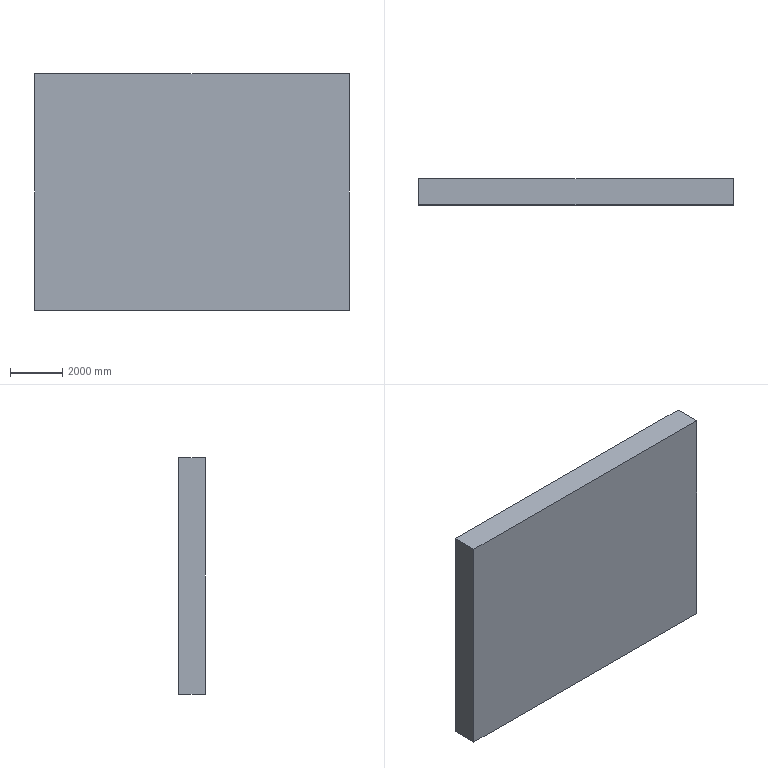Part | STEP file | Ground | 1 solid | 15 faces | box 12000 x 1000 x 9000 mm | volume 101165700000 mm3 | plane 15
STEP:
#1=CARTESIAN_POINT('',(-2380.,1000.,-2660.));
#2=VERTEX_POINT('',#1);
#3=CARTESIAN_POINT('',(-2380.,1000.,-950.));
#4=VERTEX_POINT('',#3);
#5=CARTESIAN_POINT('',(-2380.,1000.,2660.));
#6=DIRECTION('',(0.,0.,1.));
#7=VECTOR('',#6,1000.);
#8=LINE('',#5,#7);
#9=EDGE_CURVE('',#2,#4,#8,.T.);
#10=ORIENTED_EDGE('',*,*,#9,.T.);
#11=CARTESIAN_POINT('',(-2380.,455.,-950.));
#12=VERTEX_POINT('',#11);
#13=CARTESIAN_POINT('',(-2380.,-1692.091,-950.));
#14=DIRECTION('',(0.,1.,0.));
#15=VECTOR('',#14,1000.);
#16=LINE('',#13,#15);
#17=EDGE_CURVE('',#12,#4,#16,.T.);
#18=ORIENTED_EDGE('',*,*,#17,.F.);
#19=CARTESIAN_POINT('',(-2380.,455.,-2660.));
#20=VERTEX_POINT('',#19);
#21=CARTESIAN_POINT('',(-2380.,455.,2660.));
#22=DIRECTION('',(0.,0.,1.));
#23=VECTOR('',#22,1000.);
#24=LINE('',#21,#23);
#25=EDGE_CURVE('',#20,#12,#24,.T.);
#26=ORIENTED_EDGE('',*,*,#25,.F.);
#27=CARTESIAN_POINT('',(-2380.,455.,-2660.));
#28=DIRECTION('',(0.,1.,0.));
#29=VECTOR('',#28,1000.);
#30=LINE('',#27,#29);
#31=EDGE_CURVE('',#20,#2,#30,.T.);
#32=ORIENTED_EDGE('',*,*,#31,.T.);
#33=EDGE_LOOP('',(#10,#18,#26,#32));
#34=FACE_OUTER_BOUND('',#33,.T.);
#35=CARTESIAN_POINT('',(-2380.,455.,2660.));
#36=DIRECTION('',(-1.,0.,0.));
#37=DIRECTION('',(0.,0.,1.));
#38=AXIS2_PLACEMENT_3D('',#35,#36,#37);
#39=PLANE('',#38);
#40=ADVANCED_FACE('',(#34),#39,.F.);
#41=CARTESIAN_POINT('',(6000.,0.,4500.));
#42=VERTEX_POINT('',#41);
#43=CARTESIAN_POINT('',(6000.,0.,-4500.));
#44=VERTEX_POINT('',#43);
#45=CARTESIAN_POINT('',(6000.,0.,-4500.));
#46=DIRECTION('',(0.,0.,-1.));
#47=VECTOR('',#46,1000.);
#48=LINE('',#45,#47);
#49=EDGE_CURVE('',#42,#44,#48,.T.);
#50=ORIENTED_EDGE('',*,*,#49,.T.);
#51=CARTESIAN_POINT('',(6000.,1000.,-4500.));
#52=VERTEX_POINT('',#51);
#53=CARTESIAN_POINT('',(6000.,1000.,-4500.));
#54=DIRECTION('',(0.,-1.,0.));
#55=VECTOR('',#54,1000.);
#56=LINE('',#53,#55);
#57=EDGE_CURVE('',#52,#44,#56,.T.);
#58=ORIENTED_EDGE('',*,*,#57,.F.);
#59=CARTESIAN_POINT('',(6000.,1000.,4500.));
#60=VERTEX_POINT('',#59);
#61=CARTESIAN_POINT('',(6000.,1000.,-4500.));
#62=DIRECTION('',(0.,0.,-1.));
#63=VECTOR('',#62,1000.);
#64=LINE('',#61,#63);
#65=EDGE_CURVE('',#60,#52,#64,.T.);
#66=ORIENTED_EDGE('',*,*,#65,.F.);
#67=CARTESIAN_POINT('',(6000.,1000.,4500.));
#68=DIRECTION('',(0.,-1.,0.));
#69=VECTOR('',#68,1000.);
#70=LINE('',#67,#69);
#71=EDGE_CURVE('',#60,#42,#70,.T.);
#72=ORIENTED_EDGE('',*,*,#71,.T.);
#73=EDGE_LOOP('',(#50,#58,#66,#72));
#74=FACE_OUTER_BOUND('',#73,.T.);
#75=CARTESIAN_POINT('',(6000.,1000.,-4500.));
#76=DIRECTION('',(-1.,0.,0.));
#77=DIRECTION('',(0.,0.,1.));
#78=AXIS2_PLACEMENT_3D('',#75,#76,#77);
#79=PLANE('',#78);
#80=ADVANCED_FACE('',(#74),#79,.F.);
#81=CARTESIAN_POINT('',(-6000.,0.,-4500.));
#82=VERTEX_POINT('',#81);
#83=CARTESIAN_POINT('',(-6000.,0.,-4500.));
#84=DIRECTION('',(-1.,0.,0.));
#85=VECTOR('',#84,1000.);
#86=LINE('',#83,#85);
#87=EDGE_CURVE('',#44,#82,#86,.T.);
#88=ORIENTED_EDGE('',*,*,#87,.T.);
#89=CARTESIAN_POINT('',(-6000.,1000.,-4500.));
#90=VERTEX_POINT('',#89);
#91=CARTESIAN_POINT('',(-6000.,1000.,-4500.));
#92=DIRECTION('',(0.,-1.,0.));
#93=VECTOR('',#92,1000.);
#94=LINE('',#91,#93);
#95=EDGE_CURVE('',#90,#82,#94,.T.);
#96=ORIENTED_EDGE('',*,*,#95,.F.);
#97=CARTESIAN_POINT('',(-6000.,1000.,-4500.));
#98=DIRECTION('',(-1.,0.,0.));
#99=VECTOR('',#98,1000.);
#100=LINE('',#97,#99);
#101=EDGE_CURVE('',#52,#90,#100,.T.);
#102=ORIENTED_EDGE('',*,*,#101,.F.);
#103=ORIENTED_EDGE('',*,*,#57,.T.);
#104=EDGE_LOOP('',(#88,#96,#102,#103));
#105=FACE_OUTER_BOUND('',#104,.T.);
#106=CARTESIAN_POINT('',(-6000.,1000.,-4500.));
#107=DIRECTION('',(0.,0.,1.));
#108=DIRECTION('',(1.,0.,0.));
#109=AXIS2_PLACEMENT_3D('',#106,#107,#108);
#110=PLANE('',#109);
#111=ADVANCED_FACE('',(#105),#110,.F.);
#112=CARTESIAN_POINT('',(-6000.,0.,4500.));
#113=VERTEX_POINT('',#112);
#114=CARTESIAN_POINT('',(-6000.,0.,-4500.));
#115=DIRECTION('',(0.,0.,1.));
#116=VECTOR('',#115,1000.);
#117=LINE('',#114,#116);
#118=EDGE_CURVE('',#82,#113,#117,.T.);
#119=ORIENTED_EDGE('',*,*,#118,.T.);
#120=CARTESIAN_POINT('',(-6000.,1000.,4500.));
#121=VERTEX_POINT('',#120);
#122=CARTESIAN_POINT('',(-6000.,1000.,4500.));
#123=DIRECTION('',(0.,-1.,0.));
#124=VECTOR('',#123,1000.);
#125=LINE('',#122,#124);
#126=EDGE_CURVE('',#121,#113,#125,.T.);
#127=ORIENTED_EDGE('',*,*,#126,.F.);
#128=CARTESIAN_POINT('',(-6000.,1000.,-4500.));
#129=DIRECTION('',(0.,0.,1.));
#130=VECTOR('',#129,1000.);
#131=LINE('',#128,#130);
#132=EDGE_CURVE('',#90,#121,#131,.T.);
#133=ORIENTED_EDGE('',*,*,#132,.F.);
#134=ORIENTED_EDGE('',*,*,#95,.T.);
#135=EDGE_LOOP('',(#119,#127,#133,#134));
#136=FACE_OUTER_BOUND('',#135,.T.);
#137=CARTESIAN_POINT('',(-6000.,1000.,-4500.));
#138=DIRECTION('',(1.,0.,0.));
#139=DIRECTION('',(0.,0.,-1.));
#140=AXIS2_PLACEMENT_3D('',#137,#138,#139);
#141=PLANE('',#140);
#142=ADVANCED_FACE('',(#136),#141,.F.);
#143=CARTESIAN_POINT('',(-6000.,0.,4500.));
#144=DIRECTION('',(1.,0.,0.));
#145=VECTOR('',#144,1000.);
#146=LINE('',#143,#145);
#147=EDGE_CURVE('',#113,#42,#146,.T.);
#148=ORIENTED_EDGE('',*,*,#147,.T.);
#149=ORIENTED_EDGE('',*,*,#71,.F.);
#150=CARTESIAN_POINT('',(-6000.,1000.,4500.));
#151=DIRECTION('',(1.,0.,0.));
#152=VECTOR('',#151,1000.);
#153=LINE('',#150,#152);
#154=EDGE_CURVE('',#121,#60,#153,.T.);
#155=ORIENTED_EDGE('',*,*,#154,.F.);
#156=ORIENTED_EDGE('',*,*,#126,.T.);
#157=EDGE_LOOP('',(#148,#149,#155,#156));
#158=FACE_OUTER_BOUND('',#157,.T.);
#159=CARTESIAN_POINT('',(-6000.,1000.,4500.));
#160=DIRECTION('',(0.,0.,-1.));
#161=DIRECTION('',(-1.,0.,0.));
#162=AXIS2_PLACEMENT_3D('',#159,#160,#161);
#163=PLANE('',#162);
#164=ADVANCED_FACE('',(#158),#163,.F.);
#165=CARTESIAN_POINT('',(-3380.,1000.,-950.));
#166=VERTEX_POINT('',#165);
#167=CARTESIAN_POINT('',(-2380.,1000.,-950.));
#168=DIRECTION('',(-1.,0.,0.));
#169=VECTOR('',#168,1000.);
#170=LINE('',#167,#169);
#171=EDGE_CURVE('',#4,#166,#170,.T.);
#172=ORIENTED_EDGE('',*,*,#171,.F.);
#173=ORIENTED_EDGE('',*,*,#9,.F.);
#174=CARTESIAN_POINT('',(-380.,1000.,-2660.));
#175=VERTEX_POINT('',#174);
#176=CARTESIAN_POINT('',(-2380.,1000.,-2660.));
#177=DIRECTION('',(-1.,0.,0.));
#178=VECTOR('',#177,1000.);
#179=LINE('',#176,#178);
#180=EDGE_CURVE('',#175,#2,#179,.T.);
#181=ORIENTED_EDGE('',*,*,#180,.F.);
#182=CARTESIAN_POINT('',(-380.,1000.,2660.));
#183=VERTEX_POINT('',#182);
#184=CARTESIAN_POINT('',(-380.,1000.,-2660.));
#185=DIRECTION('',(0.,0.,-1.));
#186=VECTOR('',#185,1000.);
#187=LINE('',#184,#186);
#188=EDGE_CURVE('',#183,#175,#187,.T.);
#189=ORIENTED_EDGE('',*,*,#188,.F.);
#190=CARTESIAN_POINT('',(-2380.,1000.,2660.));
#191=VERTEX_POINT('',#190);
#192=CARTESIAN_POINT('',(-380.,1000.,2660.));
#193=DIRECTION('',(1.,0.,0.));
#194=VECTOR('',#193,1000.);
#195=LINE('',#192,#194);
#196=EDGE_CURVE('',#191,#183,#195,.T.);
#197=ORIENTED_EDGE('',*,*,#196,.F.);
#198=CARTESIAN_POINT('',(-2380.,1000.,950.));
#199=VERTEX_POINT('',#198);
#200=CARTESIAN_POINT('',(-2380.,1000.,2660.));
#201=DIRECTION('',(0.,0.,1.));
#202=VECTOR('',#201,1000.);
#203=LINE('',#200,#202);
#204=EDGE_CURVE('',#199,#191,#203,.T.);
#205=ORIENTED_EDGE('',*,*,#204,.F.);
#206=CARTESIAN_POINT('',(-3380.,1000.,950.));
#207=VERTEX_POINT('',#206);
#208=CARTESIAN_POINT('',(-3380.,1000.,950.));
#209=DIRECTION('',(1.,0.,0.));
#210=VECTOR('',#209,1000.);
#211=LINE('',#208,#210);
#212=EDGE_CURVE('',#207,#199,#211,.T.);
#213=ORIENTED_EDGE('',*,*,#212,.F.);
#214=CARTESIAN_POINT('',(-3380.,1000.,-950.));
#215=DIRECTION('',(0.,0.,1.));
#216=VECTOR('',#215,1000.);
#217=LINE('',#214,#216);
#218=EDGE_CURVE('',#166,#207,#217,.T.);
#219=ORIENTED_EDGE('',*,*,#218,.F.);
#220=EDGE_LOOP('',(#172,#173,#181,#189,#197,#205,#213,#219));
#221=FACE_BOUND('',#220,.T.);
#222=ORIENTED_EDGE('',*,*,#65,.T.);
#223=ORIENTED_EDGE('',*,*,#101,.T.);
#224=ORIENTED_EDGE('',*,*,#132,.T.);
#225=ORIENTED_EDGE('',*,*,#154,.T.);
#226=EDGE_LOOP('',(#222,#223,#224,#225));
#227=FACE_OUTER_BOUND('',#226,.T.);
#228=CARTESIAN_POINT('',(0.,1000.,0.));
#229=DIRECTION('',(0.,1.,0.));
#230=DIRECTION('',(0.,0.,1.));
#231=AXIS2_PLACEMENT_3D('',#228,#229,#230);
#232=PLANE('',#231);
#233=ADVANCED_FACE('',(#221,#227),#232,.T.);
#234=ORIENTED_EDGE('',*,*,#49,.F.);
#235=ORIENTED_EDGE('',*,*,#147,.F.);
#236=ORIENTED_EDGE('',*,*,#118,.F.);
#237=ORIENTED_EDGE('',*,*,#87,.F.);
#238=EDGE_LOOP('',(#234,#235,#236,#237));
#239=FACE_OUTER_BOUND('',#238,.T.);
#240=CARTESIAN_POINT('',(0.,0.,0.));
#241=DIRECTION('',(0.,1.,0.));
#242=DIRECTION('',(0.,0.,1.));
#243=AXIS2_PLACEMENT_3D('',#240,#241,#242);
#244=PLANE('',#243);
#245=ADVANCED_FACE('',(#239),#244,.F.);
#246=ORIENTED_EDGE('',*,*,#180,.T.);
#247=ORIENTED_EDGE('',*,*,#31,.F.);
#248=CARTESIAN_POINT('',(-380.,455.,-2660.));
#249=VERTEX_POINT('',#248);
#250=CARTESIAN_POINT('',(-2380.,455.,-2660.));
#251=DIRECTION('',(-1.,0.,0.));
#252=VECTOR('',#251,1000.);
#253=LINE('',#250,#252);
#254=EDGE_CURVE('',#249,#20,#253,.T.);
#255=ORIENTED_EDGE('',*,*,#254,.F.);
#256=CARTESIAN_POINT('',(-380.,455.,-2660.));
#257=DIRECTION('',(0.,1.,0.));
#258=VECTOR('',#257,1000.);
#259=LINE('',#256,#258);
#260=EDGE_CURVE('',#249,#175,#259,.T.);
#261=ORIENTED_EDGE('',*,*,#260,.T.);
#262=EDGE_LOOP('',(#246,#247,#255,#261));
#263=FACE_OUTER_BOUND('',#262,.T.);
#264=CARTESIAN_POINT('',(-2380.,455.,-2660.));
#265=DIRECTION('',(0.,0.,-1.));
#266=DIRECTION('',(-1.,0.,0.));
#267=AXIS2_PLACEMENT_3D('',#264,#265,#266);
#268=PLANE('',#267);
#269=ADVANCED_FACE('',(#263),#268,.F.);
#270=ORIENTED_EDGE('',*,*,#188,.T.);
#271=ORIENTED_EDGE('',*,*,#260,.F.);
#272=CARTESIAN_POINT('',(-380.,455.,2660.));
#273=VERTEX_POINT('',#272);
#274=CARTESIAN_POINT('',(-380.,455.,-2660.));
#275=DIRECTION('',(0.,0.,-1.));
#276=VECTOR('',#275,1000.);
#277=LINE('',#274,#276);
#278=EDGE_CURVE('',#273,#249,#277,.T.);
#279=ORIENTED_EDGE('',*,*,#278,.F.);
#280=CARTESIAN_POINT('',(-380.,455.,2660.));
#281=DIRECTION('',(0.,1.,0.));
#282=VECTOR('',#281,1000.);
#283=LINE('',#280,#282);
#284=EDGE_CURVE('',#273,#183,#283,.T.);
#285=ORIENTED_EDGE('',*,*,#284,.T.);
#286=EDGE_LOOP('',(#270,#271,#279,#285));
#287=FACE_OUTER_BOUND('',#286,.T.);
#288=CARTESIAN_POINT('',(-380.,455.,-2660.));
#289=DIRECTION('',(1.,0.,0.));
#290=DIRECTION('',(0.,0.,-1.));
#291=AXIS2_PLACEMENT_3D('',#288,#289,#290);
#292=PLANE('',#291);
#293=ADVANCED_FACE('',(#287),#292,.F.);
#294=ORIENTED_EDGE('',*,*,#196,.T.);
#295=ORIENTED_EDGE('',*,*,#284,.F.);
#296=CARTESIAN_POINT('',(-2380.,455.,2660.));
#297=VERTEX_POINT('',#296);
#298=CARTESIAN_POINT('',(-380.,455.,2660.));
#299=DIRECTION('',(1.,0.,0.));
#300=VECTOR('',#299,1000.);
#301=LINE('',#298,#300);
#302=EDGE_CURVE('',#297,#273,#301,.T.);
#303=ORIENTED_EDGE('',*,*,#302,.F.);
#304=CARTESIAN_POINT('',(-2380.,455.,2660.));
#305=DIRECTION('',(0.,1.,0.));
#306=VECTOR('',#305,1000.);
#307=LINE('',#304,#306);
#308=EDGE_CURVE('',#297,#191,#307,.T.);
#309=ORIENTED_EDGE('',*,*,#308,.T.);
#310=EDGE_LOOP('',(#294,#295,#303,#309));
#311=FACE_OUTER_BOUND('',#310,.T.);
#312=CARTESIAN_POINT('',(-380.,455.,2660.));
#313=DIRECTION('',(0.,0.,1.));
#314=DIRECTION('',(1.,0.,0.));
#315=AXIS2_PLACEMENT_3D('',#312,#313,#314);
#316=PLANE('',#315);
#317=ADVANCED_FACE('',(#311),#316,.F.);
#318=CARTESIAN_POINT('',(-2380.,455.,950.));
#319=VERTEX_POINT('',#318);
#320=CARTESIAN_POINT('',(-2380.,455.,2660.));
#321=DIRECTION('',(0.,0.,1.));
#322=VECTOR('',#321,1000.);
#323=LINE('',#320,#322);
#324=EDGE_CURVE('',#319,#297,#323,.T.);
#325=ORIENTED_EDGE('',*,*,#324,.F.);
#326=CARTESIAN_POINT('',(-2380.,-1692.091,950.));
#327=DIRECTION('',(0.,1.,0.));
#328=VECTOR('',#327,1000.);
#329=LINE('',#326,#328);
#330=EDGE_CURVE('',#319,#199,#329,.T.);
#331=ORIENTED_EDGE('',*,*,#330,.T.);
#332=ORIENTED_EDGE('',*,*,#204,.T.);
#333=ORIENTED_EDGE('',*,*,#308,.F.);
#334=EDGE_LOOP('',(#325,#331,#332,#333));
#335=FACE_OUTER_BOUND('',#334,.T.);
#336=CARTESIAN_POINT('',(-2380.,455.,2660.));
#337=DIRECTION('',(-1.,0.,0.));
#338=DIRECTION('',(0.,0.,1.));
#339=AXIS2_PLACEMENT_3D('',#336,#337,#338);
#340=PLANE('',#339);
#341=ADVANCED_FACE('',(#335),#340,.F.);
#342=ORIENTED_EDGE('',*,*,#254,.T.);
#343=ORIENTED_EDGE('',*,*,#25,.T.);
#344=CARTESIAN_POINT('',(-3380.,455.,-950.));
#345=VERTEX_POINT('',#344);
#346=CARTESIAN_POINT('',(-2380.,455.,-950.));
#347=DIRECTION('',(-1.,0.,0.));
#348=VECTOR('',#347,1000.);
#349=LINE('',#346,#348);
#350=EDGE_CURVE('',#12,#345,#349,.T.);
#351=ORIENTED_EDGE('',*,*,#350,.T.);
#352=CARTESIAN_POINT('',(-3380.,455.,950.));
#353=VERTEX_POINT('',#352);
#354=CARTESIAN_POINT('',(-3380.,455.,-950.));
#355=DIRECTION('',(0.,0.,1.));
#356=VECTOR('',#355,1000.);
#357=LINE('',#354,#356);
#358=EDGE_CURVE('',#345,#353,#357,.T.);
#359=ORIENTED_EDGE('',*,*,#358,.T.);
#360=CARTESIAN_POINT('',(-3380.,455.,950.));
#361=DIRECTION('',(1.,0.,0.));
#362=VECTOR('',#361,1000.);
#363=LINE('',#360,#362);
#364=EDGE_CURVE('',#353,#319,#363,.T.);
#365=ORIENTED_EDGE('',*,*,#364,.T.);
#366=ORIENTED_EDGE('',*,*,#324,.T.);
#367=ORIENTED_EDGE('',*,*,#302,.T.);
#368=ORIENTED_EDGE('',*,*,#278,.T.);
#369=EDGE_LOOP('',(#342,#343,#351,#359,#365,#366,#367,#368));
#370=FACE_OUTER_BOUND('',#369,.T.);
#371=CARTESIAN_POINT('',(0.,455.,0.));
#372=DIRECTION('',(0.,-1.,0.));
#373=DIRECTION('',(0.,0.,-1.));
#374=AXIS2_PLACEMENT_3D('',#371,#372,#373);
#375=PLANE('',#374);
#376=ADVANCED_FACE('',(#370),#375,.F.);
#377=ORIENTED_EDGE('',*,*,#17,.T.);
#378=ORIENTED_EDGE('',*,*,#171,.T.);
#379=CARTESIAN_POINT('',(-3380.,-1692.091,-950.));
#380=DIRECTION('',(0.,1.,0.));
#381=VECTOR('',#380,1000.);
#382=LINE('',#379,#381);
#383=EDGE_CURVE('',#345,#166,#382,.T.);
#384=ORIENTED_EDGE('',*,*,#383,.F.);
#385=ORIENTED_EDGE('',*,*,#350,.F.);
#386=EDGE_LOOP('',(#377,#378,#384,#385));
#387=FACE_OUTER_BOUND('',#386,.T.);
#388=CARTESIAN_POINT('',(-2380.,-1692.091,-950.));
#389=DIRECTION('',(0.,0.,-1.));
#390=DIRECTION('',(-1.,0.,0.));
#391=AXIS2_PLACEMENT_3D('',#388,#389,#390);
#392=PLANE('',#391);
#393=ADVANCED_FACE('',(#387),#392,.F.);
#394=ORIENTED_EDGE('',*,*,#383,.T.);
#395=ORIENTED_EDGE('',*,*,#218,.T.);
#396=CARTESIAN_POINT('',(-3380.,-1692.091,950.));
#397=DIRECTION('',(0.,1.,0.));
#398=VECTOR('',#397,1000.);
#399=LINE('',#396,#398);
#400=EDGE_CURVE('',#353,#207,#399,.T.);
#401=ORIENTED_EDGE('',*,*,#400,.F.);
#402=ORIENTED_EDGE('',*,*,#358,.F.);
#403=EDGE_LOOP('',(#394,#395,#401,#402));
#404=FACE_OUTER_BOUND('',#403,.T.);
#405=CARTESIAN_POINT('',(-3380.,-1692.091,-950.));
#406=DIRECTION('',(-1.,0.,0.));
#407=DIRECTION('',(0.,0.,1.));
#408=AXIS2_PLACEMENT_3D('',#405,#406,#407);
#409=PLANE('',#408);
#410=ADVANCED_FACE('',(#404),#409,.F.);
#411=ORIENTED_EDGE('',*,*,#400,.T.);
#412=ORIENTED_EDGE('',*,*,#212,.T.);
#413=ORIENTED_EDGE('',*,*,#330,.F.);
#414=ORIENTED_EDGE('',*,*,#364,.F.);
#415=EDGE_LOOP('',(#411,#412,#413,#414));
#416=FACE_OUTER_BOUND('',#415,.T.);
#417=CARTESIAN_POINT('',(-3380.,-1692.091,950.));
#418=DIRECTION('',(0.,0.,1.));
#419=DIRECTION('',(1.,0.,0.));
#420=AXIS2_PLACEMENT_3D('',#417,#418,#419);
#421=PLANE('',#420);
#422=ADVANCED_FACE('',(#416),#421,.F.);
#423=CLOSED_SHELL('',(#40,#80,#111,#142,#164,#233,#245,#269,#293,#317,#341,#376,#393,#410,#422));
#424=MANIFOLD_SOLID_BREP('',#423);
#425=CARTESIAN_POINT('',(0.,0.,0.));
#426=DIRECTION('',(0.,0.,1.));
#427=DIRECTION('',(1.,0.,0.));
#428=AXIS2_PLACEMENT_3D('',#425,#426,#427);
#429=(LENGTH_UNIT()NAMED_UNIT(*)SI_UNIT(.MILLI.,.METRE.));
#430=UNCERTAINTY_MEASURE_WITH_UNIT(LENGTH_MEASURE(0.00001),#429,'','');
#431=(NAMED_UNIT(*)PLANE_ANGLE_UNIT()SI_UNIT($,.RADIAN.));
#432=(NAMED_UNIT(*)SI_UNIT($,.STERADIAN.)SOLID_ANGLE_UNIT());
#433=(GEOMETRIC_REPRESENTATION_CONTEXT(3)GLOBAL_UNCERTAINTY_ASSIGNED_CONTEXT((#430))GLOBAL_UNIT_ASSIGNED_CONTEXT((#429,#431,#432))REPRESENTATION_CONTEXT('',''));
#434=ADVANCED_BREP_SHAPE_REPRESENTATION('',(#424,#428),#433);